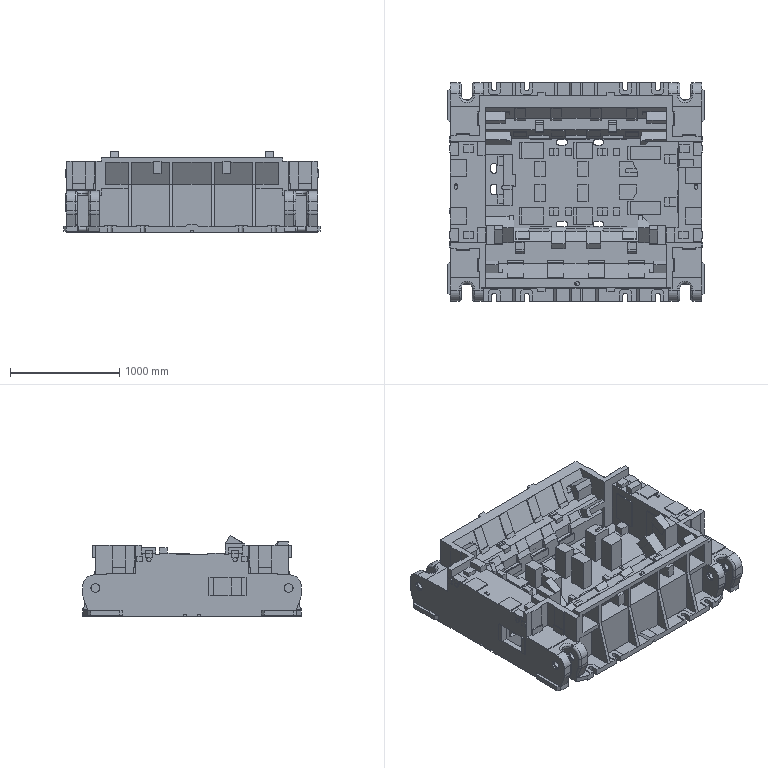Part | NX | features solid 2 | 1 solid | 1892 faces | box 2350 x 2000 x 740.801 mm | volume 792324677 mm3 | plane 1560 | cylinder 302 | torus 28 | cone 2 | commonest cylinder face diameters 40 x94 83 x48 70 x30 60 x24 80 x22 79 x16